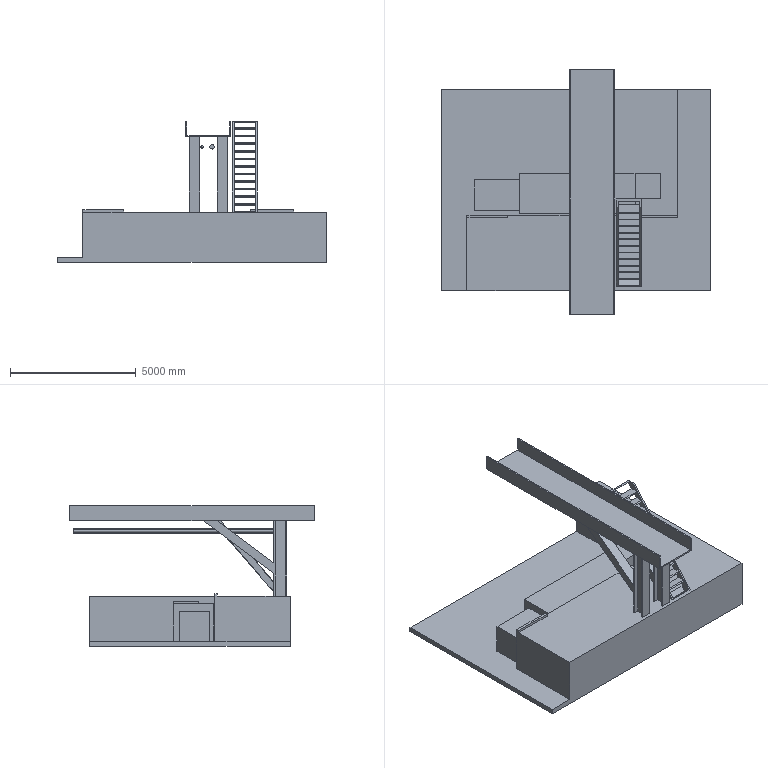Part | NX | features BREP 3 | 3 solids | 134 faces | box 10700 x 9738 x 5600 mm | volume 99535175681 mm3 | plane 130 | cylinder 4 | commonest cylinder face diameters 100 x2 180 x2